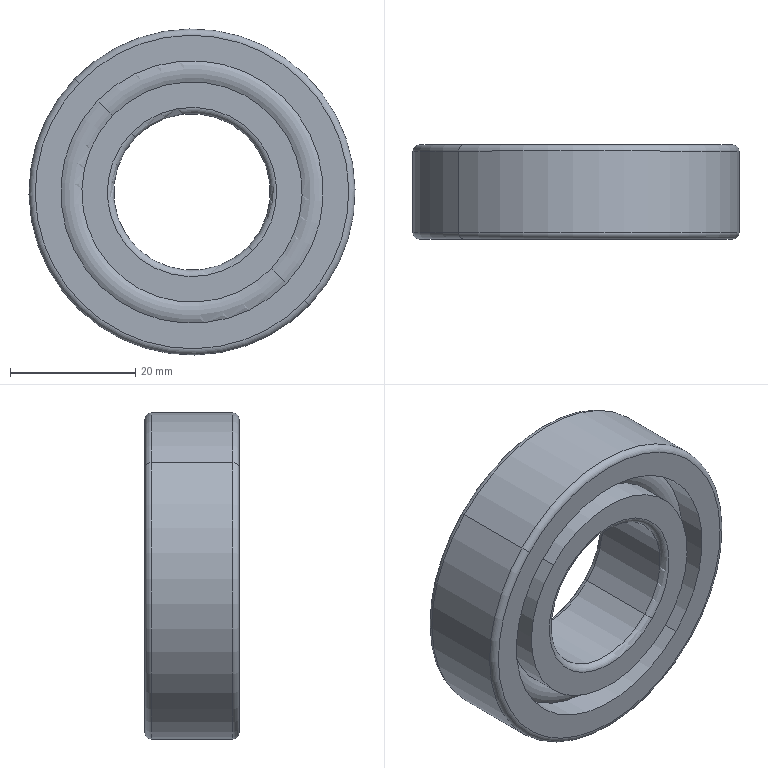Part | SolidWorks | features BaseBody 1 | 1 solid | 28 faces | box 52 x 15 x 52 mm | volume 20902 mm3 | cylinder 12 | torus 12 | plane 4 | commonest cylinder face diameters 35.125 x4 41.875 x4 25 x2 52 x2
STEP:
#1=CARTESIAN_POINT('',(502.537,830.896,-422.623));
#2=VERTEX_POINT('',#1);
#3=CARTESIAN_POINT('',(539.925,830.896,-458.763));
#4=VERTEX_POINT('',#3);
#5=CARTESIAN_POINT('',(521.231,830.896,-440.693));
#6=DIRECTION('',(0.,-1.,0.));
#7=DIRECTION('',(-0.719,0.,0.695));
#8=AXIS2_PLACEMENT_3D('',#5,#6,#7);
#9=CIRCLE('',#8,26.);
#10=EDGE_CURVE('',#2,#4,#9,.T.);
#11=ORIENTED_EDGE('',*,*,#10,.T.);
#12=CARTESIAN_POINT('',(539.925,817.896,-458.763));
#13=VERTEX_POINT('',#12);
#14=CARTESIAN_POINT('',(539.925,-176.32,-458.763));
#15=DIRECTION('',(0.,-1.,0.));
#16=VECTOR('',#15,1000.);
#17=LINE('',#14,#16);
#18=EDGE_CURVE('',#4,#13,#17,.T.);
#19=ORIENTED_EDGE('',*,*,#18,.T.);
#20=CARTESIAN_POINT('',(502.537,817.896,-422.623));
#21=VERTEX_POINT('',#20);
#22=CARTESIAN_POINT('',(521.231,817.896,-440.693));
#23=DIRECTION('',(0.,-1.,0.));
#24=DIRECTION('',(-0.719,0.,0.695));
#25=AXIS2_PLACEMENT_3D('',#22,#23,#24);
#26=CIRCLE('',#25,26.);
#27=EDGE_CURVE('',#21,#13,#26,.T.);
#28=ORIENTED_EDGE('',*,*,#27,.F.);
#29=CARTESIAN_POINT('',(502.537,-176.32,-422.623));
#30=DIRECTION('',(0.,-1.,0.));
#31=VECTOR('',#30,1000.);
#32=LINE('',#29,#31);
#33=EDGE_CURVE('',#2,#21,#32,.T.);
#34=ORIENTED_EDGE('',*,*,#33,.F.);
#35=EDGE_LOOP('',(#11,#19,#28,#34));
#36=FACE_OUTER_BOUND('',#35,.T.);
#37=CARTESIAN_POINT('',(521.231,-176.32,-440.693));
#38=DIRECTION('',(0.,-1.,0.));
#39=DIRECTION('',(-0.719,0.,0.695));
#40=AXIS2_PLACEMENT_3D('',#37,#38,#39);
#41=CYLINDRICAL_SURFACE('',#40,26.);
#42=ADVANCED_FACE('',(#36),#41,.T.);
#43=CARTESIAN_POINT('',(503.256,831.896,-423.318));
#44=VERTEX_POINT('',#43);
#45=CARTESIAN_POINT('',(539.206,831.896,-458.068));
#46=VERTEX_POINT('',#45);
#47=CARTESIAN_POINT('',(521.231,831.896,-440.693));
#48=DIRECTION('',(0.,-1.,0.));
#49=DIRECTION('',(-0.719,0.,0.695));
#50=AXIS2_PLACEMENT_3D('',#47,#48,#49);
#51=CIRCLE('',#50,25.);
#52=EDGE_CURVE('',#44,#46,#51,.T.);
#53=ORIENTED_EDGE('',*,*,#52,.T.);
#54=CARTESIAN_POINT('',(539.206,830.896,-458.068));
#55=DIRECTION('',(-0.695,0.,-0.719));
#56=DIRECTION('',(-0.719,0.,0.695));
#57=AXIS2_PLACEMENT_3D('',#54,#55,#56);
#58=CIRCLE('',#57,1.);
#59=EDGE_CURVE('',#46,#4,#58,.T.);
#60=ORIENTED_EDGE('',*,*,#59,.T.);
#61=ORIENTED_EDGE('',*,*,#10,.F.);
#62=CARTESIAN_POINT('',(503.256,830.896,-423.318));
#63=DIRECTION('',(0.695,0.,0.719));
#64=DIRECTION('',(0.719,0.,-0.695));
#65=AXIS2_PLACEMENT_3D('',#62,#63,#64);
#66=CIRCLE('',#65,1.);
#67=EDGE_CURVE('',#44,#2,#66,.T.);
#68=ORIENTED_EDGE('',*,*,#67,.F.);
#69=EDGE_LOOP('',(#53,#60,#61,#68));
#70=FACE_OUTER_BOUND('',#69,.T.);
#71=CARTESIAN_POINT('',(521.231,830.896,-440.693));
#72=DIRECTION('',(0.,-1.,0.));
#73=DIRECTION('',(-0.719,0.,0.695));
#74=AXIS2_PLACEMENT_3D('',#71,#72,#73);
#75=TOROIDAL_SURFACE('',#74,25.,1.);
#76=ADVANCED_FACE('',(#70),#75,.T.);
#77=CARTESIAN_POINT('',(536.285,831.896,-455.245));
#78=VERTEX_POINT('',#77);
#79=CARTESIAN_POINT('',(506.177,831.896,-426.141));
#80=VERTEX_POINT('',#79);
#81=CARTESIAN_POINT('',(521.231,831.896,-440.693));
#82=DIRECTION('',(0.,-1.,0.));
#83=DIRECTION('',(-0.719,0.,0.695));
#84=AXIS2_PLACEMENT_3D('',#81,#82,#83);
#85=CIRCLE('',#84,20.938);
#86=EDGE_CURVE('',#78,#80,#85,.T.);
#87=ORIENTED_EDGE('',*,*,#86,.F.);
#88=CARTESIAN_POINT('',(536.285,827.318,-455.245));
#89=VERTEX_POINT('',#88);
#90=CARTESIAN_POINT('',(536.285,-176.32,-455.245));
#91=DIRECTION('',(0.,-1.,0.));
#92=VECTOR('',#91,1000.);
#93=LINE('',#90,#92);
#94=EDGE_CURVE('',#78,#89,#93,.T.);
#95=ORIENTED_EDGE('',*,*,#94,.T.);
#96=CARTESIAN_POINT('',(506.177,827.318,-426.141));
#97=VERTEX_POINT('',#96);
#98=CARTESIAN_POINT('',(521.231,827.318,-440.693));
#99=DIRECTION('',(0.,-1.,0.));
#100=DIRECTION('',(-0.719,0.,0.695));
#101=AXIS2_PLACEMENT_3D('',#98,#99,#100);
#102=CIRCLE('',#101,20.938);
#103=EDGE_CURVE('',#89,#97,#102,.T.);
#104=ORIENTED_EDGE('',*,*,#103,.T.);
#105=CARTESIAN_POINT('',(506.177,-176.32,-426.141));
#106=DIRECTION('',(0.,-1.,0.));
#107=VECTOR('',#106,1000.);
#108=LINE('',#105,#107);
#109=EDGE_CURVE('',#80,#97,#108,.T.);
#110=ORIENTED_EDGE('',*,*,#109,.F.);
#111=EDGE_LOOP('',(#87,#95,#104,#110));
#112=FACE_OUTER_BOUND('',#111,.T.);
#113=CARTESIAN_POINT('',(521.231,-176.32,-440.693));
#114=DIRECTION('',(0.,-1.,0.));
#115=DIRECTION('',(-0.719,0.,0.695));
#116=AXIS2_PLACEMENT_3D('',#113,#114,#115);
#117=CYLINDRICAL_SURFACE('',#116,20.938);
#118=ADVANCED_FACE('',(#112),#117,.F.);
#119=CARTESIAN_POINT('',(508.603,827.318,-428.487));
#120=VERTEX_POINT('',#119);
#121=CARTESIAN_POINT('',(533.858,827.318,-452.899));
#122=VERTEX_POINT('',#121);
#123=CARTESIAN_POINT('',(521.231,827.318,-440.693));
#124=DIRECTION('',(0.,-1.,0.));
#125=DIRECTION('',(-0.719,0.,0.695));
#126=AXIS2_PLACEMENT_3D('',#123,#124,#125);
#127=CIRCLE('',#126,17.563);
#128=EDGE_CURVE('',#120,#122,#127,.T.);
#129=ORIENTED_EDGE('',*,*,#128,.T.);
#130=CARTESIAN_POINT('',(535.071,824.396,-454.072));
#131=DIRECTION('',(-0.695,0.,-0.719));
#132=DIRECTION('',(-0.719,0.,0.695));
#133=AXIS2_PLACEMENT_3D('',#130,#131,#132);
#134=CIRCLE('',#133,3.375);
#135=EDGE_CURVE('',#122,#89,#134,.T.);
#136=ORIENTED_EDGE('',*,*,#135,.T.);
#137=CARTESIAN_POINT('',(521.231,827.318,-440.693));
#138=DIRECTION('',(0.,-1.,0.));
#139=DIRECTION('',(-0.719,0.,0.695));
#140=AXIS2_PLACEMENT_3D('',#137,#138,#139);
#141=CIRCLE('',#140,20.938);
#142=EDGE_CURVE('',#97,#89,#141,.T.);
#143=ORIENTED_EDGE('',*,*,#142,.F.);
#144=CARTESIAN_POINT('',(507.39,824.396,-427.314));
#145=DIRECTION('',(0.695,0.,0.719));
#146=DIRECTION('',(0.719,0.,-0.695));
#147=AXIS2_PLACEMENT_3D('',#144,#145,#146);
#148=CIRCLE('',#147,3.375);
#149=EDGE_CURVE('',#120,#97,#148,.T.);
#150=ORIENTED_EDGE('',*,*,#149,.F.);
#151=EDGE_LOOP('',(#129,#136,#143,#150));
#152=FACE_OUTER_BOUND('',#151,.T.);
#153=CARTESIAN_POINT('',(521.231,824.396,-440.693));
#154=DIRECTION('',(0.,-1.,0.));
#155=DIRECTION('',(-0.719,0.,0.695));
#156=AXIS2_PLACEMENT_3D('',#153,#154,#155);
#157=TOROIDAL_SURFACE('',#156,19.25,3.375);
#158=ADVANCED_FACE('',(#152),#157,.T.);
#159=CARTESIAN_POINT('',(508.603,831.896,-428.487));
#160=VERTEX_POINT('',#159);
#161=CARTESIAN_POINT('',(533.858,831.896,-452.899));
#162=VERTEX_POINT('',#161);
#163=CARTESIAN_POINT('',(521.231,831.896,-440.693));
#164=DIRECTION('',(0.,-1.,0.));
#165=DIRECTION('',(-0.719,0.,0.695));
#166=AXIS2_PLACEMENT_3D('',#163,#164,#165);
#167=CIRCLE('',#166,17.563);
#168=EDGE_CURVE('',#160,#162,#167,.T.);
#169=ORIENTED_EDGE('',*,*,#168,.T.);
#170=CARTESIAN_POINT('',(533.858,-176.32,-452.899));
#171=DIRECTION('',(0.,-1.,0.));
#172=VECTOR('',#171,1000.);
#173=LINE('',#170,#172);
#174=EDGE_CURVE('',#162,#122,#173,.T.);
#175=ORIENTED_EDGE('',*,*,#174,.T.);
#176=ORIENTED_EDGE('',*,*,#128,.F.);
#177=CARTESIAN_POINT('',(508.603,-176.32,-428.487));
#178=DIRECTION('',(0.,-1.,0.));
#179=VECTOR('',#178,1000.);
#180=LINE('',#177,#179);
#181=EDGE_CURVE('',#160,#120,#180,.T.);
#182=ORIENTED_EDGE('',*,*,#181,.F.);
#183=EDGE_LOOP('',(#169,#175,#176,#182));
#184=FACE_OUTER_BOUND('',#183,.T.);
#185=CARTESIAN_POINT('',(521.231,-176.32,-440.693));
#186=DIRECTION('',(0.,-1.,0.));
#187=DIRECTION('',(-0.719,0.,0.695));
#188=AXIS2_PLACEMENT_3D('',#185,#186,#187);
#189=CYLINDRICAL_SURFACE('',#188,17.563);
#190=ADVANCED_FACE('',(#184),#189,.T.);
#191=CARTESIAN_POINT('',(512.243,830.896,-432.005));
#192=VERTEX_POINT('',#191);
#193=CARTESIAN_POINT('',(530.218,830.896,-449.381));
#194=VERTEX_POINT('',#193);
#195=CARTESIAN_POINT('',(521.231,830.896,-440.693));
#196=DIRECTION('',(0.,-1.,0.));
#197=DIRECTION('',(-0.719,0.,0.695));
#198=AXIS2_PLACEMENT_3D('',#195,#196,#197);
#199=CIRCLE('',#198,12.5);
#200=EDGE_CURVE('',#192,#194,#199,.T.);
#201=ORIENTED_EDGE('',*,*,#200,.T.);
#202=CARTESIAN_POINT('',(530.937,831.896,-450.076));
#203=VERTEX_POINT('',#202);
#204=CARTESIAN_POINT('',(530.937,830.896,-450.076));
#205=DIRECTION('',(-0.695,0.,-0.719));
#206=DIRECTION('',(-0.719,0.,0.695));
#207=AXIS2_PLACEMENT_3D('',#204,#205,#206);
#208=CIRCLE('',#207,1.);
#209=EDGE_CURVE('',#194,#203,#208,.T.);
#210=ORIENTED_EDGE('',*,*,#209,.T.);
#211=CARTESIAN_POINT('',(511.524,831.896,-431.31));
#212=VERTEX_POINT('',#211);
#213=CARTESIAN_POINT('',(521.231,831.896,-440.693));
#214=DIRECTION('',(0.,-1.,0.));
#215=DIRECTION('',(-0.719,0.,0.695));
#216=AXIS2_PLACEMENT_3D('',#213,#214,#215);
#217=CIRCLE('',#216,13.5);
#218=EDGE_CURVE('',#212,#203,#217,.T.);
#219=ORIENTED_EDGE('',*,*,#218,.F.);
#220=CARTESIAN_POINT('',(511.524,830.896,-431.31));
#221=DIRECTION('',(0.695,0.,0.719));
#222=DIRECTION('',(0.719,0.,-0.695));
#223=AXIS2_PLACEMENT_3D('',#220,#221,#222);
#224=CIRCLE('',#223,1.);
#225=EDGE_CURVE('',#192,#212,#224,.T.);
#226=ORIENTED_EDGE('',*,*,#225,.F.);
#227=EDGE_LOOP('',(#201,#210,#219,#226));
#228=FACE_OUTER_BOUND('',#227,.T.);
#229=CARTESIAN_POINT('',(521.231,830.896,-440.693));
#230=DIRECTION('',(0.,-1.,0.));
#231=DIRECTION('',(-0.719,0.,0.695));
#232=AXIS2_PLACEMENT_3D('',#229,#230,#231);
#233=TOROIDAL_SURFACE('',#232,13.5,1.);
#234=ADVANCED_FACE('',(#228),#233,.T.);
#235=CARTESIAN_POINT('',(521.231,830.896,-440.693));
#236=DIRECTION('',(0.,-1.,0.));
#237=DIRECTION('',(-0.719,0.,0.695));
#238=AXIS2_PLACEMENT_3D('',#235,#236,#237);
#239=CIRCLE('',#238,12.5);
#240=EDGE_CURVE('',#194,#192,#239,.T.);
#241=ORIENTED_EDGE('',*,*,#240,.F.);
#242=CARTESIAN_POINT('',(530.218,817.896,-449.381));
#243=VERTEX_POINT('',#242);
#244=CARTESIAN_POINT('',(530.218,-176.32,-449.381));
#245=DIRECTION('',(0.,-1.,0.));
#246=VECTOR('',#245,1000.);
#247=LINE('',#244,#246);
#248=EDGE_CURVE('',#194,#243,#247,.T.);
#249=ORIENTED_EDGE('',*,*,#248,.T.);
#250=CARTESIAN_POINT('',(512.243,817.896,-432.005));
#251=VERTEX_POINT('',#250);
#252=CARTESIAN_POINT('',(521.231,817.896,-440.693));
#253=DIRECTION('',(0.,-1.,0.));
#254=DIRECTION('',(-0.719,0.,0.695));
#255=AXIS2_PLACEMENT_3D('',#252,#253,#254);
#256=CIRCLE('',#255,12.5);
#257=EDGE_CURVE('',#243,#251,#256,.T.);
#258=ORIENTED_EDGE('',*,*,#257,.T.);
#259=CARTESIAN_POINT('',(512.243,-176.32,-432.005));
#260=DIRECTION('',(0.,-1.,0.));
#261=VECTOR('',#260,1000.);
#262=LINE('',#259,#261);
#263=EDGE_CURVE('',#192,#251,#262,.T.);
#264=ORIENTED_EDGE('',*,*,#263,.F.);
#265=EDGE_LOOP('',(#241,#249,#258,#264));
#266=FACE_OUTER_BOUND('',#265,.T.);
#267=CARTESIAN_POINT('',(521.231,-176.32,-440.693));
#268=DIRECTION('',(0.,-1.,0.));
#269=DIRECTION('',(-0.719,0.,0.695));
#270=AXIS2_PLACEMENT_3D('',#267,#268,#269);
#271=CYLINDRICAL_SURFACE('',#270,12.5);
#272=ADVANCED_FACE('',(#266),#271,.F.);
#273=CARTESIAN_POINT('',(511.524,816.896,-431.31));
#274=VERTEX_POINT('',#273);
#275=CARTESIAN_POINT('',(530.937,816.896,-450.076));
#276=VERTEX_POINT('',#275);
#277=CARTESIAN_POINT('',(521.231,816.896,-440.693));
#278=DIRECTION('',(0.,-1.,0.));
#279=DIRECTION('',(-0.719,0.,0.695));
#280=AXIS2_PLACEMENT_3D('',#277,#278,#279);
#281=CIRCLE('',#280,13.5);
#282=EDGE_CURVE('',#274,#276,#281,.T.);
#283=ORIENTED_EDGE('',*,*,#282,.T.);
#284=CARTESIAN_POINT('',(530.937,817.896,-450.076));
#285=DIRECTION('',(-0.695,0.,-0.719));
#286=DIRECTION('',(-0.719,0.,0.695));
#287=AXIS2_PLACEMENT_3D('',#284,#285,#286);
#288=CIRCLE('',#287,1.);
#289=EDGE_CURVE('',#276,#243,#288,.T.);
#290=ORIENTED_EDGE('',*,*,#289,.T.);
#291=CARTESIAN_POINT('',(521.231,817.896,-440.693));
#292=DIRECTION('',(0.,-1.,0.));
#293=DIRECTION('',(-0.719,0.,0.695));
#294=AXIS2_PLACEMENT_3D('',#291,#292,#293);
#295=CIRCLE('',#294,12.5);
#296=EDGE_CURVE('',#251,#243,#295,.T.);
#297=ORIENTED_EDGE('',*,*,#296,.F.);
#298=CARTESIAN_POINT('',(511.524,817.896,-431.31));
#299=DIRECTION('',(0.695,0.,0.719));
#300=DIRECTION('',(0.719,0.,-0.695));
#301=AXIS2_PLACEMENT_3D('',#298,#299,#300);
#302=CIRCLE('',#301,1.);
#303=EDGE_CURVE('',#274,#251,#302,.T.);
#304=ORIENTED_EDGE('',*,*,#303,.F.);
#305=EDGE_LOOP('',(#283,#290,#297,#304));
#306=FACE_OUTER_BOUND('',#305,.T.);
#307=CARTESIAN_POINT('',(521.231,817.896,-440.693));
#308=DIRECTION('',(0.,-1.,0.));
#309=DIRECTION('',(-0.719,0.,0.695));
#310=AXIS2_PLACEMENT_3D('',#307,#308,#309);
#311=TOROIDAL_SURFACE('',#310,13.5,1.);
#312=ADVANCED_FACE('',(#306),#311,.T.);
#313=CARTESIAN_POINT('',(508.603,821.473,-428.487));
#314=VERTEX_POINT('',#313);
#315=CARTESIAN_POINT('',(533.858,821.473,-452.899));
#316=VERTEX_POINT('',#315);
#317=CARTESIAN_POINT('',(521.231,821.473,-440.693));
#318=DIRECTION('',(0.,-1.,0.));
#319=DIRECTION('',(-0.719,0.,0.695));
#320=AXIS2_PLACEMENT_3D('',#317,#318,#319);
#321=CIRCLE('',#320,17.563);
#322=EDGE_CURVE('',#314,#316,#321,.T.);
#323=ORIENTED_EDGE('',*,*,#322,.T.);
#324=CARTESIAN_POINT('',(533.858,816.896,-452.899));
#325=VERTEX_POINT('',#324);
#326=CARTESIAN_POINT('',(533.858,-176.32,-452.899));
#327=DIRECTION('',(0.,-1.,0.));
#328=VECTOR('',#327,1000.);
#329=LINE('',#326,#328);
#330=EDGE_CURVE('',#316,#325,#329,.T.);
#331=ORIENTED_EDGE('',*,*,#330,.T.);
#332=CARTESIAN_POINT('',(508.603,816.896,-428.487));
#333=VERTEX_POINT('',#332);
#334=CARTESIAN_POINT('',(521.231,816.896,-440.693));
#335=DIRECTION('',(0.,-1.,0.));
#336=DIRECTION('',(-0.719,0.,0.695));
#337=AXIS2_PLACEMENT_3D('',#334,#335,#336);
#338=CIRCLE('',#337,17.563);
#339=EDGE_CURVE('',#333,#325,#338,.T.);
#340=ORIENTED_EDGE('',*,*,#339,.F.);
#341=CARTESIAN_POINT('',(508.603,-176.32,-428.487));
#342=DIRECTION('',(0.,-1.,0.));
#343=VECTOR('',#342,1000.);
#344=LINE('',#341,#343);
#345=EDGE_CURVE('',#314,#333,#344,.T.);
#346=ORIENTED_EDGE('',*,*,#345,.F.);
#347=EDGE_LOOP('',(#323,#331,#340,#346));
#348=FACE_OUTER_BOUND('',#347,.T.);
#349=CARTESIAN_POINT('',(521.231,-176.32,-440.693));
#350=DIRECTION('',(0.,-1.,0.));
#351=DIRECTION('',(-0.719,0.,0.695));
#352=AXIS2_PLACEMENT_3D('',#349,#350,#351);
#353=CYLINDRICAL_SURFACE('',#352,17.563);
#354=ADVANCED_FACE('',(#348),#353,.T.);
#355=CARTESIAN_POINT('',(506.177,821.473,-426.141));
#356=VERTEX_POINT('',#355);
#357=CARTESIAN_POINT('',(536.285,821.473,-455.245));
#358=VERTEX_POINT('',#357);
#359=CARTESIAN_POINT('',(521.231,821.473,-440.693));
#360=DIRECTION('',(0.,-1.,0.));
#361=DIRECTION('',(-0.719,0.,0.695));
#362=AXIS2_PLACEMENT_3D('',#359,#360,#361);
#363=CIRCLE('',#362,20.938);
#364=EDGE_CURVE('',#356,#358,#363,.T.);
#365=ORIENTED_EDGE('',*,*,#364,.T.);
#366=CARTESIAN_POINT('',(535.071,824.396,-454.072));
#367=DIRECTION('',(-0.695,0.,-0.719));
#368=DIRECTION('',(-0.719,0.,0.695));
#369=AXIS2_PLACEMENT_3D('',#366,#367,#368);
#370=CIRCLE('',#369,3.375);
#371=EDGE_CURVE('',#358,#316,#370,.T.);
#372=ORIENTED_EDGE('',*,*,#371,.T.);
#373=ORIENTED_EDGE('',*,*,#322,.F.);
#374=CARTESIAN_POINT('',(507.39,824.396,-427.314));
#375=DIRECTION('',(0.695,0.,0.719));
#376=DIRECTION('',(0.719,0.,-0.695));
#377=AXIS2_PLACEMENT_3D('',#374,#375,#376);
#378=CIRCLE('',#377,3.375);
#379=EDGE_CURVE('',#356,#314,#378,.T.);
#380=ORIENTED_EDGE('',*,*,#379,.F.);
#381=EDGE_LOOP('',(#365,#372,#373,#380));
#382=FACE_OUTER_BOUND('',#381,.T.);
#383=CARTESIAN_POINT('',(521.231,824.396,-440.693));
#384=DIRECTION('',(0.,-1.,0.));
#385=DIRECTION('',(-0.719,0.,0.695));
#386=AXIS2_PLACEMENT_3D('',#383,#384,#385);
#387=TOROIDAL_SURFACE('',#386,19.25,3.375);
#388=ADVANCED_FACE('',(#382),#387,.T.);
#389=CARTESIAN_POINT('',(521.231,821.473,-440.693));
#390=DIRECTION('',(0.,-1.,0.));
#391=DIRECTION('',(-0.719,0.,0.695));
#392=AXIS2_PLACEMENT_3D('',#389,#390,#391);
#393=CIRCLE('',#392,20.938);
#394=EDGE_CURVE('',#358,#356,#393,.T.);
#395=ORIENTED_EDGE('',*,*,#394,.F.);
#396=CARTESIAN_POINT('',(536.285,816.896,-455.245));
#397=VERTEX_POINT('',#396);
#398=CARTESIAN_POINT('',(536.285,-176.32,-455.245));
#399=DIRECTION('',(0.,-1.,0.));
#400=VECTOR('',#399,1000.);
#401=LINE('',#398,#400);
#402=EDGE_CURVE('',#358,#397,#401,.T.);
#403=ORIENTED_EDGE('',*,*,#402,.T.);
#404=CARTESIAN_POINT('',(506.177,816.896,-426.141));
#405=VERTEX_POINT('',#404);
#406=CARTESIAN_POINT('',(521.231,816.896,-440.693));
#407=DIRECTION('',(0.,-1.,0.));
#408=DIRECTION('',(-0.719,0.,0.695));
#409=AXIS2_PLACEMENT_3D('',#406,#407,#408);
#410=CIRCLE('',#409,20.938);
#411=EDGE_CURVE('',#397,#405,#410,.T.);
#412=ORIENTED_EDGE('',*,*,#411,.T.);
#413=CARTESIAN_POINT('',(506.177,-176.32,-426.141));
#414=DIRECTION('',(0.,-1.,0.));
#415=VECTOR('',#414,1000.);
#416=LINE('',#413,#415);
#417=EDGE_CURVE('',#356,#405,#416,.T.);
#418=ORIENTED_EDGE('',*,*,#417,.F.);
#419=EDGE_LOOP('',(#395,#403,#412,#418));
#420=FACE_OUTER_BOUND('',#419,.T.);
#421=CARTESIAN_POINT('',(521.231,-176.32,-440.693));
#422=DIRECTION('',(0.,-1.,0.));
#423=DIRECTION('',(-0.719,0.,0.695));
#424=AXIS2_PLACEMENT_3D('',#421,#422,#423);
#425=CYLINDRICAL_SURFACE('',#424,20.938);
#426=ADVANCED_FACE('',(#420),#425,.F.);
#427=ORIENTED_EDGE('',*,*,#27,.T.);
#428=CARTESIAN_POINT('',(539.206,816.896,-458.068));
#429=VERTEX_POINT('',#428);
#430=CARTESIAN_POINT('',(539.206,817.896,-458.068));
#431=DIRECTION('',(-0.695,0.,-0.719));
#432=DIRECTION('',(-0.719,0.,0.695));
#433=AXIS2_PLACEMENT_3D('',#430,#431,#432);
#434=CIRCLE('',#433,1.);
#435=EDGE_CURVE('',#13,#429,#434,.T.);
#436=ORIENTED_EDGE('',*,*,#435,.T.);
#437=CARTESIAN_POINT('',(503.256,816.896,-423.318));
#438=VERTEX_POINT('',#437);
#439=CARTESIAN_POINT('',(521.231,816.896,-440.693));
#440=DIRECTION('',(0.,-1.,0.));
#441=DIRECTION('',(-0.719,0.,0.695));
#442=AXIS2_PLACEMENT_3D('',#439,#440,#441);
#443=CIRCLE('',#442,25.);
#444=EDGE_CURVE('',#438,#429,#443,.T.);
#445=ORIENTED_EDGE('',*,*,#444,.F.);
#446=CARTESIAN_POINT('',(503.256,817.896,-423.318));
#447=DIRECTION('',(0.695,0.,0.719));
#448=DIRECTION('',(0.719,0.,-0.695));
#449=AXIS2_PLACEMENT_3D('',#446,#447,#448);
#450=CIRCLE('',#449,1.);
#451=EDGE_CURVE('',#21,#438,#450,.T.);
#452=ORIENTED_EDGE('',*,*,#451,.F.);
#453=EDGE_LOOP('',(#427,#436,#445,#452));
#454=FACE_OUTER_BOUND('',#453,.T.);
#455=CARTESIAN_POINT('',(521.231,817.896,-440.693));
#456=DIRECTION('',(0.,-1.,0.));
#457=DIRECTION('',(-0.719,0.,0.695));
#458=AXIS2_PLACEMENT_3D('',#455,#456,#457);
#459=TOROIDAL_SURFACE('',#458,25.,1.);
#460=ADVANCED_FACE('',(#454),#459,.T.);
#461=ORIENTED_EDGE('',*,*,#435,.F.);
#462=CARTESIAN_POINT('',(521.231,817.896,-440.693));
#463=DIRECTION('',(0.,-1.,0.));
#464=DIRECTION('',(-0.719,0.,0.695));
#465=AXIS2_PLACEMENT_3D('',#462,#463,#464);
#466=CIRCLE('',#465,26.);
#467=EDGE_CURVE('',#13,#21,#466,.T.);
#468=ORIENTED_EDGE('',*,*,#467,.T.);
#469=ORIENTED_EDGE('',*,*,#451,.T.);
#470=CARTESIAN_POINT('',(521.231,816.896,-440.693));
#471=DIRECTION('',(0.,-1.,0.));
#472=DIRECTION('',(-0.719,0.,0.695));
#473=AXIS2_PLACEMENT_3D('',#470,#471,#472);
#474=CIRCLE('',#473,25.);
#475=EDGE_CURVE('',#429,#438,#474,.T.);
#476=ORIENTED_EDGE('',*,*,#475,.F.);
#477=EDGE_LOOP('',(#461,#468,#469,#476));
#478=FACE_OUTER_BOUND('',#477,.T.);
#479=CARTESIAN_POINT('',(521.231,817.896,-440.693));
#480=DIRECTION('',(0.,-1.,0.));
#481=DIRECTION('',(-0.719,0.,0.695));
#482=AXIS2_PLACEMENT_3D('',#479,#480,#481);
#483=TOROIDAL_SURFACE('',#482,25.,1.);
#484=ADVANCED_FACE('',(#478),#483,.T.);
#485=CARTESIAN_POINT('',(521.231,816.896,-440.693));
#486=DIRECTION('',(0.,-1.,0.));
#487=DIRECTION('',(-0.719,0.,0.695));
#488=AXIS2_PLACEMENT_3D('',#485,#486,#487);
#489=CIRCLE('',#488,20.938);
#490=EDGE_CURVE('',#405,#397,#489,.T.);
#491=ORIENTED_EDGE('',*,*,#490,.F.);
#492=ORIENTED_EDGE('',*,*,#411,.F.);
#493=EDGE_LOOP('',(#491,#492));
#494=FACE_BOUND('',#493,.T.);
#495=ORIENTED_EDGE('',*,*,#444,.T.);
#496=ORIENTED_EDGE('',*,*,#475,.T.);
#497=EDGE_LOOP('',(#495,#496));
#498=FACE_OUTER_BOUND('',#497,.T.);
#499=CARTESIAN_POINT('',(503.855,816.896,-458.668));
#500=DIRECTION('',(0.,1.,0.));
#501=DIRECTION('',(0.719,0.,-0.695));
#502=AXIS2_PLACEMENT_3D('',#499,#500,#501);
#503=PLANE('',#502);
#504=ADVANCED_FACE('',(#494,#498),#503,.F.);
#505=ORIENTED_EDGE('',*,*,#402,.F.);
#506=ORIENTED_EDGE('',*,*,#364,.F.);
#507=ORIENTED_EDGE('',*,*,#417,.T.);
#508=ORIENTED_EDGE('',*,*,#490,.T.);
#509=EDGE_LOOP('',(#505,#506,#507,#508));
#510=FACE_OUTER_BOUND('',#509,.T.);
#511=CARTESIAN_POINT('',(521.231,-176.32,-440.693));
#512=DIRECTION('',(0.,-1.,0.));
#513=DIRECTION('',(-0.719,0.,0.695));
#514=AXIS2_PLACEMENT_3D('',#511,#512,#513);
#515=CYLINDRICAL_SURFACE('',#514,20.938);
#516=ADVANCED_FACE('',(#510),#515,.F.);
#517=ORIENTED_EDGE('',*,*,#371,.F.);
#518=ORIENTED_EDGE('',*,*,#394,.T.);
#519=ORIENTED_EDGE('',*,*,#379,.T.);
#520=CARTESIAN_POINT('',(521.231,821.473,-440.693));
#521=DIRECTION('',(0.,-1.,0.));
#522=DIRECTION('',(-0.719,0.,0.695));
#523=AXIS2_PLACEMENT_3D('',#520,#521,#522);
#524=CIRCLE('',#523,17.563);
#525=EDGE_CURVE('',#316,#314,#524,.T.);
#526=ORIENTED_EDGE('',*,*,#525,.F.);
#527=EDGE_LOOP('',(#517,#518,#519,#526));
#528=FACE_OUTER_BOUND('',#527,.T.);
#529=CARTESIAN_POINT('',(521.231,824.396,-440.693));
#530=DIRECTION('',(0.,-1.,0.));
#531=DIRECTION('',(-0.719,0.,0.695));
#532=AXIS2_PLACEMENT_3D('',#529,#530,#531);
#533=TOROIDAL_SURFACE('',#532,19.25,3.375);
#534=ADVANCED_FACE('',(#528),#533,.T.);
#535=ORIENTED_EDGE('',*,*,#330,.F.);
#536=ORIENTED_EDGE('',*,*,#525,.T.);
#537=ORIENTED_EDGE('',*,*,#345,.T.);
#538=CARTESIAN_POINT('',(521.231,816.896,-440.693));
#539=DIRECTION('',(0.,-1.,0.));
#540=DIRECTION('',(-0.719,0.,0.695));
#541=AXIS2_PLACEMENT_3D('',#538,#539,#540);
#542=CIRCLE('',#541,17.563);
#543=EDGE_CURVE('',#325,#333,#542,.T.);
#544=ORIENTED_EDGE('',*,*,#543,.F.);
#545=EDGE_LOOP('',(#535,#536,#537,#544));
#546=FACE_OUTER_BOUND('',#545,.T.);
#547=CARTESIAN_POINT('',(521.231,-176.32,-440.693));
#548=DIRECTION('',(0.,-1.,0.));
#549=DIRECTION('',(-0.719,0.,0.695));
#550=AXIS2_PLACEMENT_3D('',#547,#548,#549);
#551=CYLINDRICAL_SURFACE('',#550,17.563);
#552=ADVANCED_FACE('',(#546),#551,.T.);
#553=ORIENTED_EDGE('',*,*,#282,.F.);
#554=CARTESIAN_POINT('',(521.231,816.896,-440.693));
#555=DIRECTION('',(0.,-1.,0.));
#556=DIRECTION('',(-0.719,0.,0.695));
#557=AXIS2_PLACEMENT_3D('',#554,#555,#556);
#558=CIRCLE('',#557,13.5);
#559=EDGE_CURVE('',#276,#274,#558,.T.);
#560=ORIENTED_EDGE('',*,*,#559,.F.);
#561=EDGE_LOOP('',(#553,#560));
#562=FACE_BOUND('',#561,.T.);
#563=ORIENTED_EDGE('',*,*,#339,.T.);
#564=ORIENTED_EDGE('',*,*,#543,.T.);
#565=EDGE_LOOP('',(#563,#564));
#566=FACE_OUTER_BOUND('',#565,.T.);
#567=CARTESIAN_POINT('',(509.025,816.896,-453.32));
#568=DIRECTION('',(0.,1.,0.));
#569=DIRECTION('',(0.719,0.,-0.695));
#570=AXIS2_PLACEMENT_3D('',#567,#568,#569);
#571=PLANE('',#570);
#572=ADVANCED_FACE('',(#562,#566),#571,.F.);
#573=ORIENTED_EDGE('',*,*,#289,.F.);
#574=ORIENTED_EDGE('',*,*,#559,.T.);
#575=ORIENTED_EDGE('',*,*,#303,.T.);
#576=ORIENTED_EDGE('',*,*,#257,.F.);
#577=EDGE_LOOP('',(#573,#574,#575,#576));
#578=FACE_OUTER_BOUND('',#577,.T.);
#579=CARTESIAN_POINT('',(521.231,817.896,-440.693));
#580=DIRECTION('',(0.,-1.,0.));
#581=DIRECTION('',(-0.719,0.,0.695));
#582=AXIS2_PLACEMENT_3D('',#579,#580,#581);
#583=TOROIDAL_SURFACE('',#582,13.5,1.);
#584=ADVANCED_FACE('',(#578),#583,.T.);
#585=ORIENTED_EDGE('',*,*,#248,.F.);
#586=ORIENTED_EDGE('',*,*,#200,.F.);
#587=ORIENTED_EDGE('',*,*,#263,.T.);
#588=ORIENTED_EDGE('',*,*,#296,.T.);
#589=EDGE_LOOP('',(#585,#586,#587,#588));
#590=FACE_OUTER_BOUND('',#589,.T.);
#591=CARTESIAN_POINT('',(521.231,-176.32,-440.693));
#592=DIRECTION('',(0.,-1.,0.));
#593=DIRECTION('',(-0.719,0.,0.695));
#594=AXIS2_PLACEMENT_3D('',#591,#592,#593);
#595=CYLINDRICAL_SURFACE('',#594,12.5);
#596=ADVANCED_FACE('',(#590),#595,.F.);
#597=ORIENTED_EDGE('',*,*,#209,.F.);
#598=ORIENTED_EDGE('',*,*,#240,.T.);
#599=ORIENTED_EDGE('',*,*,#225,.T.);
#600=CARTESIAN_POINT('',(521.231,831.896,-440.693));
#601=DIRECTION('',(0.,-1.,0.));
#602=DIRECTION('',(-0.719,0.,0.695));
#603=AXIS2_PLACEMENT_3D('',#600,#601,#602);
#604=CIRCLE('',#603,13.5);
#605=EDGE_CURVE('',#203,#212,#604,.T.);
#606=ORIENTED_EDGE('',*,*,#605,.F.);
#607=EDGE_LOOP('',(#597,#598,#599,#606));
#608=FACE_OUTER_BOUND('',#607,.T.);
#609=CARTESIAN_POINT('',(521.231,830.896,-440.693));
#610=DIRECTION('',(0.,-1.,0.));
#611=DIRECTION('',(-0.719,0.,0.695));
#612=AXIS2_PLACEMENT_3D('',#609,#610,#611);
#613=TOROIDAL_SURFACE('',#612,13.5,1.);
#614=ADVANCED_FACE('',(#608),#613,.T.);
#615=ORIENTED_EDGE('',*,*,#168,.F.);
#616=CARTESIAN_POINT('',(521.231,831.896,-440.693));
#617=DIRECTION('',(0.,-1.,0.));
#618=DIRECTION('',(-0.719,0.,0.695));
#619=AXIS2_PLACEMENT_3D('',#616,#617,#618);
#620=CIRCLE('',#619,17.563);
#621=EDGE_CURVE('',#162,#160,#620,.T.);
#622=ORIENTED_EDGE('',*,*,#621,.F.);
#623=EDGE_LOOP('',(#615,#622));
#624=FACE_OUTER_BOUND('',#623,.T.);
#625=ORIENTED_EDGE('',*,*,#218,.T.);
#626=ORIENTED_EDGE('',*,*,#605,.T.);
#627=EDGE_LOOP('',(#625,#626));
#628=FACE_BOUND('',#627,.T.);
#629=CARTESIAN_POINT('',(509.025,831.896,-453.32));
#630=DIRECTION('',(0.,-1.,0.));
#631=DIRECTION('',(-0.719,0.,0.695));
#632=AXIS2_PLACEMENT_3D('',#629,#630,#631);
#633=PLANE('',#632);
#634=ADVANCED_FACE('',(#624,#628),#633,.F.);
#635=ORIENTED_EDGE('',*,*,#174,.F.);
#636=ORIENTED_EDGE('',*,*,#621,.T.);
#637=ORIENTED_EDGE('',*,*,#181,.T.);
#638=CARTESIAN_POINT('',(521.231,827.318,-440.693));
#639=DIRECTION('',(0.,-1.,0.));
#640=DIRECTION('',(-0.719,0.,0.695));
#641=AXIS2_PLACEMENT_3D('',#638,#639,#640);
#642=CIRCLE('',#641,17.563);
#643=EDGE_CURVE('',#122,#120,#642,.T.);
#644=ORIENTED_EDGE('',*,*,#643,.F.);
#645=EDGE_LOOP('',(#635,#636,#637,#644));
#646=FACE_OUTER_BOUND('',#645,.T.);
#647=CARTESIAN_POINT('',(521.231,-176.32,-440.693));
#648=DIRECTION('',(0.,-1.,0.));
#649=DIRECTION('',(-0.719,0.,0.695));
#650=AXIS2_PLACEMENT_3D('',#647,#648,#649);
#651=CYLINDRICAL_SURFACE('',#650,17.563);
#652=ADVANCED_FACE('',(#646),#651,.T.);
#653=ORIENTED_EDGE('',*,*,#135,.F.);
#654=ORIENTED_EDGE('',*,*,#643,.T.);
#655=ORIENTED_EDGE('',*,*,#149,.T.);
#656=ORIENTED_EDGE('',*,*,#103,.F.);
#657=EDGE_LOOP('',(#653,#654,#655,#656));
#658=FACE_OUTER_BOUND('',#657,.T.);
#659=CARTESIAN_POINT('',(521.231,824.396,-440.693));
#660=DIRECTION('',(0.,-1.,0.));
#661=DIRECTION('',(-0.719,0.,0.695));
#662=AXIS2_PLACEMENT_3D('',#659,#660,#661);
#663=TOROIDAL_SURFACE('',#662,19.25,3.375);
#664=ADVANCED_FACE('',(#658),#663,.T.);
#665=ORIENTED_EDGE('',*,*,#94,.F.);
#666=CARTESIAN_POINT('',(521.231,831.896,-440.693));
#667=DIRECTION('',(0.,-1.,0.));
#668=DIRECTION('',(-0.719,0.,0.695));
#669=AXIS2_PLACEMENT_3D('',#666,#667,#668);
#670=CIRCLE('',#669,20.938);
#671=EDGE_CURVE('',#80,#78,#670,.T.);
#672=ORIENTED_EDGE('',*,*,#671,.F.);
#673=ORIENTED_EDGE('',*,*,#109,.T.);
#674=ORIENTED_EDGE('',*,*,#142,.T.);
#675=EDGE_LOOP('',(#665,#672,#673,#674));
#676=FACE_OUTER_BOUND('',#675,.T.);
#677=CARTESIAN_POINT('',(521.231,-176.32,-440.693));
#678=DIRECTION('',(0.,-1.,0.));
#679=DIRECTION('',(-0.719,0.,0.695));
#680=AXIS2_PLACEMENT_3D('',#677,#678,#679);
#681=CYLINDRICAL_SURFACE('',#680,20.938);
#682=ADVANCED_FACE('',(#676),#681,.F.);
#683=ORIENTED_EDGE('',*,*,#52,.F.);
#684=CARTESIAN_POINT('',(521.231,831.896,-440.693));
#685=DIRECTION('',(0.,-1.,0.));
#686=DIRECTION('',(-0.719,0.,0.695));
#687=AXIS2_PLACEMENT_3D('',#684,#685,#686);
#688=CIRCLE('',#687,25.);
#689=EDGE_CURVE('',#46,#44,#688,.T.);
#690=ORIENTED_EDGE('',*,*,#689,.F.);
#691=EDGE_LOOP('',(#683,#690));
#692=FACE_OUTER_BOUND('',#691,.T.);
#693=ORIENTED_EDGE('',*,*,#671,.T.);
#694=ORIENTED_EDGE('',*,*,#86,.T.);
#695=EDGE_LOOP('',(#693,#694));
#696=FACE_BOUND('',#695,.T.);
#697=CARTESIAN_POINT('',(503.855,831.896,-458.668));
#698=DIRECTION('',(0.,-1.,0.));
#699=DIRECTION('',(-0.719,0.,0.695));
#700=AXIS2_PLACEMENT_3D('',#697,#698,#699);
#701=PLANE('',#700);
#702=ADVANCED_FACE('',(#692,#696),#701,.F.);
#703=ORIENTED_EDGE('',*,*,#59,.F.);
#704=ORIENTED_EDGE('',*,*,#689,.T.);
#705=ORIENTED_EDGE('',*,*,#67,.T.);
#706=CARTESIAN_POINT('',(521.231,830.896,-440.693));
#707=DIRECTION('',(0.,-1.,0.));
#708=DIRECTION('',(-0.719,0.,0.695));
#709=AXIS2_PLACEMENT_3D('',#706,#707,#708);
#710=CIRCLE('',#709,26.);
#711=EDGE_CURVE('',#4,#2,#710,.T.);
#712=ORIENTED_EDGE('',*,*,#711,.F.);
#713=EDGE_LOOP('',(#703,#704,#705,#712));
#714=FACE_OUTER_BOUND('',#713,.T.);
#715=CARTESIAN_POINT('',(521.231,830.896,-440.693));
#716=DIRECTION('',(0.,-1.,0.));
#717=DIRECTION('',(-0.719,0.,0.695));
#718=AXIS2_PLACEMENT_3D('',#715,#716,#717);
#719=TOROIDAL_SURFACE('',#718,25.,1.);
#720=ADVANCED_FACE('',(#714),#719,.T.);
#721=ORIENTED_EDGE('',*,*,#18,.F.);
#722=ORIENTED_EDGE('',*,*,#711,.T.);
#723=ORIENTED_EDGE('',*,*,#33,.T.);
#724=ORIENTED_EDGE('',*,*,#467,.F.);
#725=EDGE_LOOP('',(#721,#722,#723,#724));
#726=FACE_OUTER_BOUND('',#725,.T.);
#727=CARTESIAN_POINT('',(521.231,-176.32,-440.693));
#728=DIRECTION('',(0.,-1.,0.));
#729=DIRECTION('',(-0.719,0.,0.695));
#730=AXIS2_PLACEMENT_3D('',#727,#728,#729);
#731=CYLINDRICAL_SURFACE('',#730,26.);
#732=ADVANCED_FACE('',(#726),#731,.T.);
#733=CLOSED_SHELL('',(#42,#76,#118,#158,#190,#234,#272,#312,#354,#388,#426,#460,#484,#504,#516,#534,#552,#572,#584,#596,#614,#634,#652,#664,#682,#702,#720,#732));
#734=MANIFOLD_SOLID_BREP('',#733);
#735=CARTESIAN_POINT('',(0.,0.,0.));
#736=DIRECTION('',(0.,0.,1.));
#737=DIRECTION('',(1.,0.,0.));
#738=AXIS2_PLACEMENT_3D('',#735,#736,#737);
#739=(LENGTH_UNIT()NAMED_UNIT(*)SI_UNIT(.MILLI.,.METRE.));
#740=UNCERTAINTY_MEASURE_WITH_UNIT(LENGTH_MEASURE(0.00001),#739,'','');
#741=(NAMED_UNIT(*)PLANE_ANGLE_UNIT()SI_UNIT($,.RADIAN.));
#742=(NAMED_UNIT(*)SI_UNIT($,.STERADIAN.)SOLID_ANGLE_UNIT());
#743=(GEOMETRIC_REPRESENTATION_CONTEXT(3)GLOBAL_UNCERTAINTY_ASSIGNED_CONTEXT((#740))GLOBAL_UNIT_ASSIGNED_CONTEXT((#739,#741,#742))REPRESENTATION_CONTEXT('',''));
#744=ADVANCED_BREP_SHAPE_REPRESENTATION('',(#734,#738),#743);